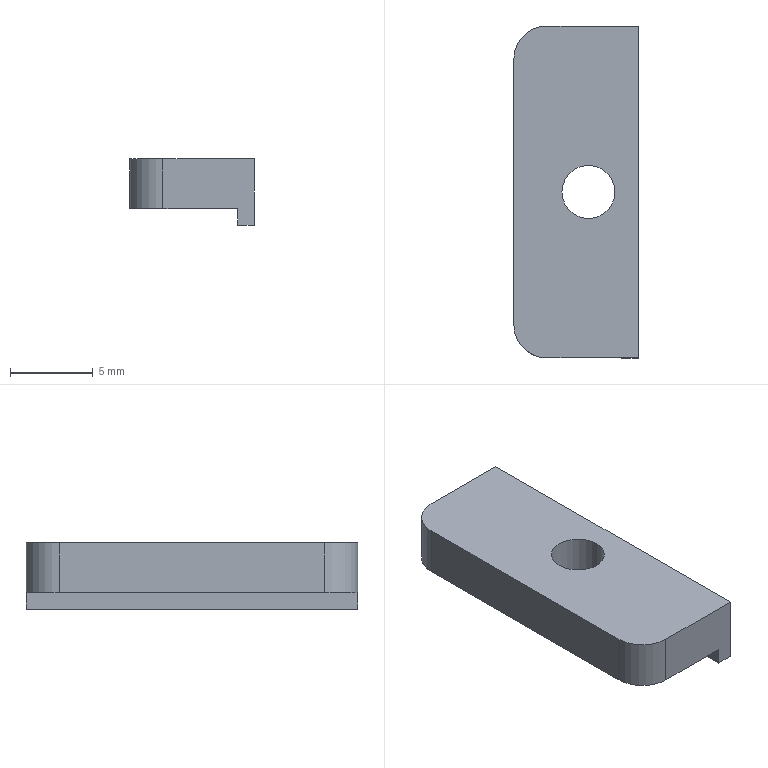Part | STEP file | PN_0043 Mount electronic clip pressure block A | 1 solid | 12 faces | box 7.5 x 20 x 4 mm | volume 440.722 mm3 | plane 8 | cylinder 4 | commonest cylinder face diameters 3.2 x2 4 x2
STEP:
#1=CARTESIAN_POINT('',(0.,0.,0.));
#2=DIRECTION('',(0.,0.,1.));
#3=DIRECTION('',(1.,0.,0.));
#4=AXIS2_PLACEMENT_3D('',#1,#2,#3);
#5=CARTESIAN_POINT('',(2.35,0.,1.));
#6=VERTEX_POINT('',#5);
#7=CARTESIAN_POINT('',(2.35,0.,4.));
#8=VERTEX_POINT('',#7);
#9=CARTESIAN_POINT('',(2.35,0.,4.));
#10=DIRECTION('',(0.,0.,1.));
#11=VECTOR('',#10,1.);
#12=LINE('',#9,#11);
#13=CARTESIAN_POINT('',(0.75,0.,4.));
#14=DIRECTION('',(0.,0.,1.));
#15=DIRECTION('',(1.,0.,0.));
#16=AXIS2_PLACEMENT_3D('',#13,#14,#15);
#17=CYLINDRICAL_SURFACE('',#16,1.6);
#18=CARTESIAN_POINT('',(6.283,0.));
#19=DIRECTION('',(0.,1.));
#20=VECTOR('',#19,1.);
#21=LINE('',#18,#20);
#22=(GEOMETRIC_REPRESENTATION_CONTEXT(2)PARAMETRIC_REPRESENTATION_CONTEXT()REPRESENTATION_CONTEXT('',''));
#23=DEFINITIONAL_REPRESENTATION('',(#21),#22);
#24=PCURVE('',#17,#23);
#25=CARTESIAN_POINT('',(0.75,0.,4.));
#26=DIRECTION('',(0.,0.,1.));
#27=DIRECTION('',(1.,0.,0.));
#28=AXIS2_PLACEMENT_3D('',#25,#26,#27);
#29=CYLINDRICAL_SURFACE('',#28,1.6);
#30=CARTESIAN_POINT('',(0.,0.));
#31=DIRECTION('',(0.,1.));
#32=VECTOR('',#31,1.);
#33=LINE('',#30,#32);
#34=(GEOMETRIC_REPRESENTATION_CONTEXT(2)PARAMETRIC_REPRESENTATION_CONTEXT()REPRESENTATION_CONTEXT('',''));
#35=DEFINITIONAL_REPRESENTATION('',(#33),#34);
#36=PCURVE('',#29,#35);
#37=SURFACE_CURVE('',#12,(#24,#36),.PCURVE_S1.);
#38=EDGE_CURVE('',#6,#8,#37,.T.);
#39=ORIENTED_EDGE('',*,*,#38,.T.);
#40=CARTESIAN_POINT('',(-0.85,0.,4.));
#41=VERTEX_POINT('',#40);
#42=CARTESIAN_POINT('',(0.75,0.,4.));
#43=DIRECTION('',(0.,0.,1.));
#44=DIRECTION('',(1.,0.,0.));
#45=AXIS2_PLACEMENT_3D('',#42,#43,#44);
#46=CIRCLE('',#45,1.6);
#47=CARTESIAN_POINT('',(0.,0.));
#48=DIRECTION('',(1.,0.));
#49=VECTOR('',#48,1.);
#50=LINE('',#47,#49);
#51=(GEOMETRIC_REPRESENTATION_CONTEXT(2)PARAMETRIC_REPRESENTATION_CONTEXT()REPRESENTATION_CONTEXT('',''));
#52=DEFINITIONAL_REPRESENTATION('',(#50),#51);
#53=PCURVE('',#17,#52);
#54=CARTESIAN_POINT('',(0.,0.,4.));
#55=DIRECTION('',(0.,0.,-1.));
#56=DIRECTION('',(-1.,0.,0.));
#57=AXIS2_PLACEMENT_3D('',#54,#55,#56);
#58=PLANE('',#57);
#59=CARTESIAN_POINT('',(-2.35,0.));
#60=CARTESIAN_POINT('',(-2.35,2.771));
#61=CARTESIAN_POINT('',(0.05,1.386));
#62=CARTESIAN_POINT('',(2.45,0.));
#63=CARTESIAN_POINT('',(0.05,-1.386));
#64=CARTESIAN_POINT('',(-2.35,-2.771));
#65=CARTESIAN_POINT('',(-2.35,0.));
#66=(BOUNDED_CURVE()B_SPLINE_CURVE(2,(#59,#60,#61,#62,#63,#64,#65),.UNSPECIFIED.,.T.,.F.)B_SPLINE_CURVE_WITH_KNOTS((1,2,2,2,2,1),(-2.094,0.,2.094,4.189,6.283,8.378),.UNSPECIFIED.)CURVE()GEOMETRIC_REPRESENTATION_ITEM()RATIONAL_B_SPLINE_CURVE((1.,0.5,1.,0.5,1.,0.5,1.))REPRESENTATION_ITEM(''));
#67=(GEOMETRIC_REPRESENTATION_CONTEXT(2)PARAMETRIC_REPRESENTATION_CONTEXT()REPRESENTATION_CONTEXT('',''));
#68=DEFINITIONAL_REPRESENTATION('',(#66),#67);
#69=PCURVE('',#58,#68);
#70=SURFACE_CURVE('',#46,(#53,#69),.PCURVE_S1.);
#71=EDGE_CURVE('',#41,#8,#70,.T.);
#72=ORIENTED_EDGE('',*,*,#71,.F.);
#73=CARTESIAN_POINT('',(-0.85,0.,1.));
#74=VERTEX_POINT('',#73);
#75=CARTESIAN_POINT('',(-0.85,0.,4.));
#76=DIRECTION('',(0.,0.,1.));
#77=VECTOR('',#76,1.);
#78=LINE('',#75,#77);
#79=CARTESIAN_POINT('',(3.142,0.));
#80=DIRECTION('',(0.,1.));
#81=VECTOR('',#80,1.);
#82=LINE('',#79,#81);
#83=(GEOMETRIC_REPRESENTATION_CONTEXT(2)PARAMETRIC_REPRESENTATION_CONTEXT()REPRESENTATION_CONTEXT('',''));
#84=DEFINITIONAL_REPRESENTATION('',(#82),#83);
#85=PCURVE('',#17,#84);
#86=CARTESIAN_POINT('',(3.142,0.));
#87=DIRECTION('',(0.,1.));
#88=VECTOR('',#87,1.);
#89=LINE('',#86,#88);
#90=(GEOMETRIC_REPRESENTATION_CONTEXT(2)PARAMETRIC_REPRESENTATION_CONTEXT()REPRESENTATION_CONTEXT('',''));
#91=DEFINITIONAL_REPRESENTATION('',(#89),#90);
#92=PCURVE('',#29,#91);
#93=SURFACE_CURVE('',#78,(#85,#92),.PCURVE_S1.);
#94=EDGE_CURVE('',#74,#41,#93,.T.);
#95=ORIENTED_EDGE('',*,*,#94,.F.);
#96=CARTESIAN_POINT('',(0.75,0.,1.));
#97=DIRECTION('',(0.,0.,1.));
#98=DIRECTION('',(1.,0.,0.));
#99=AXIS2_PLACEMENT_3D('',#96,#97,#98);
#100=CIRCLE('',#99,1.6);
#101=CARTESIAN_POINT('',(0.,-3.));
#102=DIRECTION('',(1.,0.));
#103=VECTOR('',#102,1.);
#104=LINE('',#101,#103);
#105=(GEOMETRIC_REPRESENTATION_CONTEXT(2)PARAMETRIC_REPRESENTATION_CONTEXT()REPRESENTATION_CONTEXT('',''));
#106=DEFINITIONAL_REPRESENTATION('',(#104),#105);
#107=PCURVE('',#17,#106);
#108=CARTESIAN_POINT('',(-3.75,10.,1.));
#109=DIRECTION('',(0.,0.,1.));
#110=DIRECTION('',(1.,0.,0.));
#111=AXIS2_PLACEMENT_3D('',#108,#109,#110);
#112=PLANE('',#111);
#113=CARTESIAN_POINT('',(4.5,-10.));
#114=DIRECTION('',(1.,0.));
#115=AXIS2_PLACEMENT_2D('',#113,#114);
#116=CIRCLE('',#115,1.6);
#117=(GEOMETRIC_REPRESENTATION_CONTEXT(2)PARAMETRIC_REPRESENTATION_CONTEXT()REPRESENTATION_CONTEXT('',''));
#118=DEFINITIONAL_REPRESENTATION('',(#116),#117);
#119=PCURVE('',#112,#118);
#120=SURFACE_CURVE('',#100,(#107,#119),.PCURVE_S1.);
#121=EDGE_CURVE('',#74,#6,#120,.T.);
#122=ORIENTED_EDGE('',*,*,#121,.T.);
#123=EDGE_LOOP('',(#39,#72,#95,#122));
#124=FACE_BOUND('',#123,.F.);
#125=ADVANCED_FACE('',(#124),#17,.F.);
#126=CARTESIAN_POINT('',(3.75,-10.,0.));
#127=VERTEX_POINT('',#126);
#128=CARTESIAN_POINT('',(3.75,10.,0.));
#129=VERTEX_POINT('',#128);
#130=CARTESIAN_POINT('',(3.75,-10.,0.));
#131=DIRECTION('',(0.,1.,0.));
#132=VECTOR('',#131,1.);
#133=LINE('',#130,#132);
#134=CARTESIAN_POINT('',(3.75,-10.,4.));
#135=DIRECTION('',(-1.,0.,0.));
#136=DIRECTION('',(0.,0.,1.));
#137=AXIS2_PLACEMENT_3D('',#134,#135,#136);
#138=PLANE('',#137);
#139=CARTESIAN_POINT('',(-4.,0.));
#140=DIRECTION('',(0.,1.));
#141=VECTOR('',#140,1.);
#142=LINE('',#139,#141);
#143=(GEOMETRIC_REPRESENTATION_CONTEXT(2)PARAMETRIC_REPRESENTATION_CONTEXT()REPRESENTATION_CONTEXT('',''));
#144=DEFINITIONAL_REPRESENTATION('',(#142),#143);
#145=PCURVE('',#138,#144);
#146=CARTESIAN_POINT('',(0.,0.,0.));
#147=DIRECTION('',(0.,0.,-1.));
#148=DIRECTION('',(-1.,0.,0.));
#149=AXIS2_PLACEMENT_3D('',#146,#147,#148);
#150=PLANE('',#149);
#151=CARTESIAN_POINT('',(-3.75,-10.));
#152=DIRECTION('',(0.,1.));
#153=VECTOR('',#152,1.);
#154=LINE('',#151,#153);
#155=(GEOMETRIC_REPRESENTATION_CONTEXT(2)PARAMETRIC_REPRESENTATION_CONTEXT()REPRESENTATION_CONTEXT('',''));
#156=DEFINITIONAL_REPRESENTATION('',(#154),#155);
#157=PCURVE('',#150,#156);
#158=SURFACE_CURVE('',#133,(#145,#157),.PCURVE_S1.);
#159=EDGE_CURVE('',#127,#129,#158,.T.);
#160=ORIENTED_EDGE('',*,*,#159,.T.);
#161=CARTESIAN_POINT('',(3.75,10.,4.));
#162=VERTEX_POINT('',#161);
#163=CARTESIAN_POINT('',(3.75,10.,4.));
#164=DIRECTION('',(0.,0.,-1.));
#165=VECTOR('',#164,1.);
#166=LINE('',#163,#165);
#167=CARTESIAN_POINT('',(0.,20.));
#168=DIRECTION('',(-1.,0.));
#169=VECTOR('',#168,1.);
#170=LINE('',#167,#169);
#171=(GEOMETRIC_REPRESENTATION_CONTEXT(2)PARAMETRIC_REPRESENTATION_CONTEXT()REPRESENTATION_CONTEXT('',''));
#172=DEFINITIONAL_REPRESENTATION('',(#170),#171);
#173=PCURVE('',#138,#172);
#174=CARTESIAN_POINT('',(-3.75,10.,4.));
#175=DIRECTION('',(0.,-1.,0.));
#176=DIRECTION('',(0.,0.,-1.));
#177=AXIS2_PLACEMENT_3D('',#174,#175,#176);
#178=PLANE('',#177);
#179=CARTESIAN_POINT('',(0.,7.5));
#180=DIRECTION('',(1.,0.));
#181=VECTOR('',#180,1.);
#182=LINE('',#179,#181);
#183=(GEOMETRIC_REPRESENTATION_CONTEXT(2)PARAMETRIC_REPRESENTATION_CONTEXT()REPRESENTATION_CONTEXT('',''));
#184=DEFINITIONAL_REPRESENTATION('',(#182),#183);
#185=PCURVE('',#178,#184);
#186=SURFACE_CURVE('',#166,(#173,#185),.PCURVE_S1.);
#187=EDGE_CURVE('',#162,#129,#186,.T.);
#188=ORIENTED_EDGE('',*,*,#187,.F.);
#189=CARTESIAN_POINT('',(3.75,-10.,4.));
#190=VERTEX_POINT('',#189);
#191=CARTESIAN_POINT('',(3.75,-10.,4.));
#192=DIRECTION('',(0.,1.,0.));
#193=VECTOR('',#192,1.);
#194=LINE('',#191,#193);
#195=CARTESIAN_POINT('',(0.,0.));
#196=DIRECTION('',(0.,1.));
#197=VECTOR('',#196,1.);
#198=LINE('',#195,#197);
#199=(GEOMETRIC_REPRESENTATION_CONTEXT(2)PARAMETRIC_REPRESENTATION_CONTEXT()REPRESENTATION_CONTEXT('',''));
#200=DEFINITIONAL_REPRESENTATION('',(#198),#199);
#201=PCURVE('',#138,#200);
#202=CARTESIAN_POINT('',(-3.75,-10.));
#203=DIRECTION('',(0.,1.));
#204=VECTOR('',#203,1.);
#205=LINE('',#202,#204);
#206=(GEOMETRIC_REPRESENTATION_CONTEXT(2)PARAMETRIC_REPRESENTATION_CONTEXT()REPRESENTATION_CONTEXT('',''));
#207=DEFINITIONAL_REPRESENTATION('',(#205),#206);
#208=PCURVE('',#58,#207);
#209=SURFACE_CURVE('',#194,(#201,#208),.PCURVE_S1.);
#210=EDGE_CURVE('',#190,#162,#209,.T.);
#211=ORIENTED_EDGE('',*,*,#210,.F.);
#212=CARTESIAN_POINT('',(3.75,-10.,4.));
#213=DIRECTION('',(0.,0.,-1.));
#214=VECTOR('',#213,1.);
#215=LINE('',#212,#214);
#216=CARTESIAN_POINT('',(0.,0.));
#217=DIRECTION('',(-1.,0.));
#218=VECTOR('',#217,1.);
#219=LINE('',#216,#218);
#220=(GEOMETRIC_REPRESENTATION_CONTEXT(2)PARAMETRIC_REPRESENTATION_CONTEXT()REPRESENTATION_CONTEXT('',''));
#221=DEFINITIONAL_REPRESENTATION('',(#219),#220);
#222=PCURVE('',#138,#221);
#223=CARTESIAN_POINT('',(-3.75,-10.,4.));
#224=DIRECTION('',(0.,1.,0.));
#225=DIRECTION('',(0.,0.,1.));
#226=AXIS2_PLACEMENT_3D('',#223,#224,#225);
#227=PLANE('',#226);
#228=CARTESIAN_POINT('',(0.,7.5));
#229=DIRECTION('',(-1.,0.));
#230=VECTOR('',#229,1.);
#231=LINE('',#228,#230);
#232=(GEOMETRIC_REPRESENTATION_CONTEXT(2)PARAMETRIC_REPRESENTATION_CONTEXT()REPRESENTATION_CONTEXT('',''));
#233=DEFINITIONAL_REPRESENTATION('',(#231),#232);
#234=PCURVE('',#227,#233);
#235=SURFACE_CURVE('',#215,(#222,#234),.PCURVE_S1.);
#236=EDGE_CURVE('',#190,#127,#235,.T.);
#237=ORIENTED_EDGE('',*,*,#236,.T.);
#238=EDGE_LOOP('',(#160,#188,#211,#237));
#239=FACE_BOUND('',#238,.T.);
#240=ADVANCED_FACE('',(#239),#138,.F.);
#241=CARTESIAN_POINT('',(2.75,10.,1.));
#242=VERTEX_POINT('',#241);
#243=CARTESIAN_POINT('',(-1.75,10.,1.));
#244=VERTEX_POINT('',#243);
#245=CARTESIAN_POINT('',(-3.75,10.,1.));
#246=DIRECTION('',(-1.,0.,0.));
#247=VECTOR('',#246,1.);
#248=LINE('',#245,#247);
#249=CARTESIAN_POINT('',(3.,0.));
#250=DIRECTION('',(0.,-1.));
#251=VECTOR('',#250,1.);
#252=LINE('',#249,#251);
#253=(GEOMETRIC_REPRESENTATION_CONTEXT(2)PARAMETRIC_REPRESENTATION_CONTEXT()REPRESENTATION_CONTEXT('',''));
#254=DEFINITIONAL_REPRESENTATION('',(#252),#253);
#255=PCURVE('',#178,#254);
#256=CARTESIAN_POINT('',(0.,0.));
#257=DIRECTION('',(-1.,0.));
#258=VECTOR('',#257,1.);
#259=LINE('',#256,#258);
#260=(GEOMETRIC_REPRESENTATION_CONTEXT(2)PARAMETRIC_REPRESENTATION_CONTEXT()REPRESENTATION_CONTEXT('',''));
#261=DEFINITIONAL_REPRESENTATION('',(#259),#260);
#262=PCURVE('',#112,#261);
#263=SURFACE_CURVE('',#248,(#255,#262),.PCURVE_S1.);
#264=EDGE_CURVE('',#242,#244,#263,.T.);
#265=ORIENTED_EDGE('',*,*,#264,.T.);
#266=CARTESIAN_POINT('',(-1.75,10.,4.));
#267=VERTEX_POINT('',#266);
#268=CARTESIAN_POINT('',(-1.75,10.,4.));
#269=DIRECTION('',(0.,0.,1.));
#270=VECTOR('',#269,1.);
#271=LINE('',#268,#270);
#272=CARTESIAN_POINT('',(0.,2.));
#273=DIRECTION('',(-1.,0.));
#274=VECTOR('',#273,1.);
#275=LINE('',#272,#274);
#276=(GEOMETRIC_REPRESENTATION_CONTEXT(2)PARAMETRIC_REPRESENTATION_CONTEXT()REPRESENTATION_CONTEXT('',''));
#277=DEFINITIONAL_REPRESENTATION('',(#275),#276);
#278=PCURVE('',#178,#277);
#279=CARTESIAN_POINT('',(-1.75,8.,4.));
#280=DIRECTION('',(0.,0.,-1.));
#281=DIRECTION('',(-1.,0.,0.));
#282=AXIS2_PLACEMENT_3D('',#279,#280,#281);
#283=CYLINDRICAL_SURFACE('',#282,2.);
#284=CARTESIAN_POINT('',(1.571,0.));
#285=DIRECTION('',(0.,-1.));
#286=VECTOR('',#285,1.);
#287=LINE('',#284,#286);
#288=(GEOMETRIC_REPRESENTATION_CONTEXT(2)PARAMETRIC_REPRESENTATION_CONTEXT()REPRESENTATION_CONTEXT('',''));
#289=DEFINITIONAL_REPRESENTATION('',(#287),#288);
#290=PCURVE('',#283,#289);
#291=SURFACE_CURVE('',#271,(#278,#290),.PCURVE_S1.);
#292=EDGE_CURVE('',#244,#267,#291,.T.);
#293=ORIENTED_EDGE('',*,*,#292,.T.);
#294=CARTESIAN_POINT('',(-3.75,10.,4.));
#295=DIRECTION('',(-1.,0.,0.));
#296=VECTOR('',#295,1.);
#297=LINE('',#294,#296);
#298=CARTESIAN_POINT('',(0.,0.));
#299=DIRECTION('',(0.,-1.));
#300=VECTOR('',#299,1.);
#301=LINE('',#298,#300);
#302=(GEOMETRIC_REPRESENTATION_CONTEXT(2)PARAMETRIC_REPRESENTATION_CONTEXT()REPRESENTATION_CONTEXT('',''));
#303=DEFINITIONAL_REPRESENTATION('',(#301),#302);
#304=PCURVE('',#178,#303);
#305=CARTESIAN_POINT('',(3.75,10.));
#306=DIRECTION('',(1.,0.));
#307=VECTOR('',#306,1.);
#308=LINE('',#305,#307);
#309=(GEOMETRIC_REPRESENTATION_CONTEXT(2)PARAMETRIC_REPRESENTATION_CONTEXT()REPRESENTATION_CONTEXT('',''));
#310=DEFINITIONAL_REPRESENTATION('',(#308),#309);
#311=PCURVE('',#58,#310);
#312=SURFACE_CURVE('',#297,(#304,#311),.PCURVE_S1.);
#313=EDGE_CURVE('',#162,#267,#312,.T.);
#314=ORIENTED_EDGE('',*,*,#313,.F.);
#315=ORIENTED_EDGE('',*,*,#187,.T.);
#316=CARTESIAN_POINT('',(2.75,10.,0.));
#317=VERTEX_POINT('',#316);
#318=CARTESIAN_POINT('',(-3.75,10.,0.));
#319=DIRECTION('',(-1.,0.,0.));
#320=VECTOR('',#319,1.);
#321=LINE('',#318,#320);
#322=CARTESIAN_POINT('',(4.,0.));
#323=DIRECTION('',(0.,-1.));
#324=VECTOR('',#323,1.);
#325=LINE('',#322,#324);
#326=(GEOMETRIC_REPRESENTATION_CONTEXT(2)PARAMETRIC_REPRESENTATION_CONTEXT()REPRESENTATION_CONTEXT('',''));
#327=DEFINITIONAL_REPRESENTATION('',(#325),#326);
#328=PCURVE('',#178,#327);
#329=CARTESIAN_POINT('',(3.75,10.));
#330=DIRECTION('',(1.,0.));
#331=VECTOR('',#330,1.);
#332=LINE('',#329,#331);
#333=(GEOMETRIC_REPRESENTATION_CONTEXT(2)PARAMETRIC_REPRESENTATION_CONTEXT()REPRESENTATION_CONTEXT('',''));
#334=DEFINITIONAL_REPRESENTATION('',(#332),#333);
#335=PCURVE('',#150,#334);
#336=SURFACE_CURVE('',#321,(#328,#335),.PCURVE_S1.);
#337=EDGE_CURVE('',#129,#317,#336,.T.);
#338=ORIENTED_EDGE('',*,*,#337,.T.);
#339=CARTESIAN_POINT('',(2.75,10.,0.));
#340=DIRECTION('',(0.,0.,1.));
#341=VECTOR('',#340,1.);
#342=LINE('',#339,#341);
#343=CARTESIAN_POINT('',(4.,6.5));
#344=DIRECTION('',(-1.,0.));
#345=VECTOR('',#344,1.);
#346=LINE('',#343,#345);
#347=(GEOMETRIC_REPRESENTATION_CONTEXT(2)PARAMETRIC_REPRESENTATION_CONTEXT()REPRESENTATION_CONTEXT('',''));
#348=DEFINITIONAL_REPRESENTATION('',(#346),#347);
#349=PCURVE('',#178,#348);
#350=CARTESIAN_POINT('',(2.75,10.,0.));
#351=DIRECTION('',(1.,0.,0.));
#352=DIRECTION('',(0.,0.,-1.));
#353=AXIS2_PLACEMENT_3D('',#350,#351,#352);
#354=PLANE('',#353);
#355=CARTESIAN_POINT('',(0.,0.));
#356=DIRECTION('',(-1.,0.));
#357=VECTOR('',#356,1.);
#358=LINE('',#355,#357);
#359=(GEOMETRIC_REPRESENTATION_CONTEXT(2)PARAMETRIC_REPRESENTATION_CONTEXT()REPRESENTATION_CONTEXT('',''));
#360=DEFINITIONAL_REPRESENTATION('',(#358),#359);
#361=PCURVE('',#354,#360);
#362=SURFACE_CURVE('',#342,(#349,#361),.PCURVE_S1.);
#363=EDGE_CURVE('',#317,#242,#362,.T.);
#364=ORIENTED_EDGE('',*,*,#363,.T.);
#365=EDGE_LOOP('',(#265,#293,#314,#315,#338,#364));
#366=FACE_BOUND('',#365,.T.);
#367=ADVANCED_FACE('',(#366),#178,.F.);
#368=CARTESIAN_POINT('',(-3.75,8.,4.));
#369=VERTEX_POINT('',#368);
#370=CARTESIAN_POINT('',(-3.75,-8.,4.));
#371=VERTEX_POINT('',#370);
#372=CARTESIAN_POINT('',(-3.75,-10.,4.));
#373=DIRECTION('',(0.,-1.,0.));
#374=VECTOR('',#373,1.);
#375=LINE('',#372,#374);
#376=CARTESIAN_POINT('',(-3.75,-10.,4.));
#377=DIRECTION('',(1.,0.,0.));
#378=DIRECTION('',(0.,0.,-1.));
#379=AXIS2_PLACEMENT_3D('',#376,#377,#378);
#380=PLANE('',#379);
#381=CARTESIAN_POINT('',(0.,0.));
#382=DIRECTION('',(0.,-1.));
#383=VECTOR('',#382,1.);
#384=LINE('',#381,#383);
#385=(GEOMETRIC_REPRESENTATION_CONTEXT(2)PARAMETRIC_REPRESENTATION_CONTEXT()REPRESENTATION_CONTEXT('',''));
#386=DEFINITIONAL_REPRESENTATION('',(#384),#385);
#387=PCURVE('',#380,#386);
#388=CARTESIAN_POINT('',(3.75,-10.));
#389=DIRECTION('',(0.,-1.));
#390=VECTOR('',#389,1.);
#391=LINE('',#388,#390);
#392=(GEOMETRIC_REPRESENTATION_CONTEXT(2)PARAMETRIC_REPRESENTATION_CONTEXT()REPRESENTATION_CONTEXT('',''));
#393=DEFINITIONAL_REPRESENTATION('',(#391),#392);
#394=PCURVE('',#58,#393);
#395=SURFACE_CURVE('',#375,(#387,#394),.PCURVE_S1.);
#396=EDGE_CURVE('',#369,#371,#395,.T.);
#397=ORIENTED_EDGE('',*,*,#396,.F.);
#398=CARTESIAN_POINT('',(-3.75,8.,1.));
#399=VERTEX_POINT('',#398);
#400=CARTESIAN_POINT('',(-3.75,8.,4.));
#401=DIRECTION('',(0.,0.,-1.));
#402=VECTOR('',#401,1.);
#403=LINE('',#400,#402);
#404=CARTESIAN_POINT('',(0.,18.));
#405=DIRECTION('',(1.,0.));
#406=VECTOR('',#405,1.);
#407=LINE('',#404,#406);
#408=(GEOMETRIC_REPRESENTATION_CONTEXT(2)PARAMETRIC_REPRESENTATION_CONTEXT()REPRESENTATION_CONTEXT('',''));
#409=DEFINITIONAL_REPRESENTATION('',(#407),#408);
#410=PCURVE('',#380,#409);
#411=CARTESIAN_POINT('',(0.,0.));
#412=DIRECTION('',(0.,1.));
#413=VECTOR('',#412,1.);
#414=LINE('',#411,#413);
#415=(GEOMETRIC_REPRESENTATION_CONTEXT(2)PARAMETRIC_REPRESENTATION_CONTEXT()REPRESENTATION_CONTEXT('',''));
#416=DEFINITIONAL_REPRESENTATION('',(#414),#415);
#417=PCURVE('',#283,#416);
#418=SURFACE_CURVE('',#403,(#410,#417),.PCURVE_S1.);
#419=EDGE_CURVE('',#369,#399,#418,.T.);
#420=ORIENTED_EDGE('',*,*,#419,.T.);
#421=CARTESIAN_POINT('',(-3.75,-8.,1.));
#422=VERTEX_POINT('',#421);
#423=CARTESIAN_POINT('',(-3.75,10.,1.));
#424=DIRECTION('',(0.,-1.,0.));
#425=VECTOR('',#424,1.);
#426=LINE('',#423,#425);
#427=CARTESIAN_POINT('',(3.,20.));
#428=DIRECTION('',(0.,-1.));
#429=VECTOR('',#428,1.);
#430=LINE('',#427,#429);
#431=(GEOMETRIC_REPRESENTATION_CONTEXT(2)PARAMETRIC_REPRESENTATION_CONTEXT()REPRESENTATION_CONTEXT('',''));
#432=DEFINITIONAL_REPRESENTATION('',(#430),#431);
#433=PCURVE('',#380,#432);
#434=CARTESIAN_POINT('',(0.,0.));
#435=DIRECTION('',(0.,-1.));
#436=VECTOR('',#435,1.);
#437=LINE('',#434,#436);
#438=(GEOMETRIC_REPRESENTATION_CONTEXT(2)PARAMETRIC_REPRESENTATION_CONTEXT()REPRESENTATION_CONTEXT('',''));
#439=DEFINITIONAL_REPRESENTATION('',(#437),#438);
#440=PCURVE('',#112,#439);
#441=SURFACE_CURVE('',#426,(#433,#440),.PCURVE_S1.);
#442=EDGE_CURVE('',#399,#422,#441,.T.);
#443=ORIENTED_EDGE('',*,*,#442,.T.);
#444=CARTESIAN_POINT('',(-3.75,-8.,4.));
#445=DIRECTION('',(0.,0.,1.));
#446=VECTOR('',#445,1.);
#447=LINE('',#444,#446);
#448=CARTESIAN_POINT('',(0.,2.));
#449=DIRECTION('',(-1.,0.));
#450=VECTOR('',#449,1.);
#451=LINE('',#448,#450);
#452=(GEOMETRIC_REPRESENTATION_CONTEXT(2)PARAMETRIC_REPRESENTATION_CONTEXT()REPRESENTATION_CONTEXT('',''));
#453=DEFINITIONAL_REPRESENTATION('',(#451),#452);
#454=PCURVE('',#380,#453);
#455=CARTESIAN_POINT('',(-1.75,-8.,4.));
#456=DIRECTION('',(0.,0.,-1.));
#457=DIRECTION('',(-1.,0.,0.));
#458=AXIS2_PLACEMENT_3D('',#455,#456,#457);
#459=CYLINDRICAL_SURFACE('',#458,2.);
#460=CARTESIAN_POINT('',(6.283,0.));
#461=DIRECTION('',(0.,-1.));
#462=VECTOR('',#461,1.);
#463=LINE('',#460,#462);
#464=(GEOMETRIC_REPRESENTATION_CONTEXT(2)PARAMETRIC_REPRESENTATION_CONTEXT()REPRESENTATION_CONTEXT('',''));
#465=DEFINITIONAL_REPRESENTATION('',(#463),#464);
#466=PCURVE('',#459,#465);
#467=SURFACE_CURVE('',#447,(#454,#466),.PCURVE_S1.);
#468=EDGE_CURVE('',#422,#371,#467,.T.);
#469=ORIENTED_EDGE('',*,*,#468,.T.);
#470=EDGE_LOOP('',(#397,#420,#443,#469));
#471=FACE_BOUND('',#470,.T.);
#472=ADVANCED_FACE('',(#471),#380,.F.);
#473=CARTESIAN_POINT('',(-1.75,-10.,4.));
#474=VERTEX_POINT('',#473);
#475=CARTESIAN_POINT('',(-3.75,-10.,4.));
#476=DIRECTION('',(1.,0.,0.));
#477=VECTOR('',#476,1.);
#478=LINE('',#475,#477);
#479=CARTESIAN_POINT('',(0.,0.));
#480=DIRECTION('',(0.,1.));
#481=VECTOR('',#480,1.);
#482=LINE('',#479,#481);
#483=(GEOMETRIC_REPRESENTATION_CONTEXT(2)PARAMETRIC_REPRESENTATION_CONTEXT()REPRESENTATION_CONTEXT('',''));
#484=DEFINITIONAL_REPRESENTATION('',(#482),#483);
#485=PCURVE('',#227,#484);
#486=CARTESIAN_POINT('',(3.75,-10.));
#487=DIRECTION('',(-1.,0.));
#488=VECTOR('',#487,1.);
#489=LINE('',#486,#488);
#490=(GEOMETRIC_REPRESENTATION_CONTEXT(2)PARAMETRIC_REPRESENTATION_CONTEXT()REPRESENTATION_CONTEXT('',''));
#491=DEFINITIONAL_REPRESENTATION('',(#489),#490);
#492=PCURVE('',#58,#491);
#493=SURFACE_CURVE('',#478,(#485,#492),.PCURVE_S1.);
#494=EDGE_CURVE('',#474,#190,#493,.T.);
#495=ORIENTED_EDGE('',*,*,#494,.F.);
#496=CARTESIAN_POINT('',(-1.75,-10.,1.));
#497=VERTEX_POINT('',#496);
#498=CARTESIAN_POINT('',(-1.75,-10.,4.));
#499=DIRECTION('',(0.,0.,-1.));
#500=VECTOR('',#499,1.);
#501=LINE('',#498,#500);
#502=CARTESIAN_POINT('',(0.,2.));
#503=DIRECTION('',(-1.,0.));
#504=VECTOR('',#503,1.);
#505=LINE('',#502,#504);
#506=(GEOMETRIC_REPRESENTATION_CONTEXT(2)PARAMETRIC_REPRESENTATION_CONTEXT()REPRESENTATION_CONTEXT('',''));
#507=DEFINITIONAL_REPRESENTATION('',(#505),#506);
#508=PCURVE('',#227,#507);
#509=CARTESIAN_POINT('',(4.712,0.));
#510=DIRECTION('',(0.,1.));
#511=VECTOR('',#510,1.);
#512=LINE('',#509,#511);
#513=(GEOMETRIC_REPRESENTATION_CONTEXT(2)PARAMETRIC_REPRESENTATION_CONTEXT()REPRESENTATION_CONTEXT('',''));
#514=DEFINITIONAL_REPRESENTATION('',(#512),#513);
#515=PCURVE('',#459,#514);
#516=SURFACE_CURVE('',#501,(#508,#515),.PCURVE_S1.);
#517=EDGE_CURVE('',#474,#497,#516,.T.);
#518=ORIENTED_EDGE('',*,*,#517,.T.);
#519=CARTESIAN_POINT('',(2.75,-10.,1.));
#520=VERTEX_POINT('',#519);
#521=CARTESIAN_POINT('',(-3.75,-10.,1.));
#522=DIRECTION('',(-1.,0.,0.));
#523=VECTOR('',#522,1.);
#524=LINE('',#521,#523);
#525=CARTESIAN_POINT('',(-3.,0.));
#526=DIRECTION('',(0.,-1.));
#527=VECTOR('',#526,1.);
#528=LINE('',#525,#527);
#529=(GEOMETRIC_REPRESENTATION_CONTEXT(2)PARAMETRIC_REPRESENTATION_CONTEXT()REPRESENTATION_CONTEXT('',''));
#530=DEFINITIONAL_REPRESENTATION('',(#528),#529);
#531=PCURVE('',#227,#530);
#532=CARTESIAN_POINT('',(0.,-20.));
#533=DIRECTION('',(-1.,0.));
#534=VECTOR('',#533,1.);
#535=LINE('',#532,#534);
#536=(GEOMETRIC_REPRESENTATION_CONTEXT(2)PARAMETRIC_REPRESENTATION_CONTEXT()REPRESENTATION_CONTEXT('',''));
#537=DEFINITIONAL_REPRESENTATION('',(#535),#536);
#538=PCURVE('',#112,#537);
#539=SURFACE_CURVE('',#524,(#531,#538),.PCURVE_S1.);
#540=EDGE_CURVE('',#520,#497,#539,.T.);
#541=ORIENTED_EDGE('',*,*,#540,.F.);
#542=CARTESIAN_POINT('',(2.75,-10.,0.));
#543=VERTEX_POINT('',#542);
#544=CARTESIAN_POINT('',(2.75,-10.,0.));
#545=DIRECTION('',(0.,0.,1.));
#546=VECTOR('',#545,1.);
#547=LINE('',#544,#546);
#548=CARTESIAN_POINT('',(-4.,6.5));
#549=DIRECTION('',(1.,0.));
#550=VECTOR('',#549,1.);
#551=LINE('',#548,#550);
#552=(GEOMETRIC_REPRESENTATION_CONTEXT(2)PARAMETRIC_REPRESENTATION_CONTEXT()REPRESENTATION_CONTEXT('',''));
#553=DEFINITIONAL_REPRESENTATION('',(#551),#552);
#554=PCURVE('',#227,#553);
#555=CARTESIAN_POINT('',(0.,-20.));
#556=DIRECTION('',(-1.,0.));
#557=VECTOR('',#556,1.);
#558=LINE('',#555,#557);
#559=(GEOMETRIC_REPRESENTATION_CONTEXT(2)PARAMETRIC_REPRESENTATION_CONTEXT()REPRESENTATION_CONTEXT('',''));
#560=DEFINITIONAL_REPRESENTATION('',(#558),#559);
#561=PCURVE('',#354,#560);
#562=SURFACE_CURVE('',#547,(#554,#561),.PCURVE_S1.);
#563=EDGE_CURVE('',#543,#520,#562,.T.);
#564=ORIENTED_EDGE('',*,*,#563,.F.);
#565=CARTESIAN_POINT('',(-3.75,-10.,0.));
#566=DIRECTION('',(1.,0.,0.));
#567=VECTOR('',#566,1.);
#568=LINE('',#565,#567);
#569=CARTESIAN_POINT('',(-4.,0.));
#570=DIRECTION('',(0.,1.));
#571=VECTOR('',#570,1.);
#572=LINE('',#569,#571);
#573=(GEOMETRIC_REPRESENTATION_CONTEXT(2)PARAMETRIC_REPRESENTATION_CONTEXT()REPRESENTATION_CONTEXT('',''));
#574=DEFINITIONAL_REPRESENTATION('',(#572),#573);
#575=PCURVE('',#227,#574);
#576=CARTESIAN_POINT('',(3.75,-10.));
#577=DIRECTION('',(-1.,0.));
#578=VECTOR('',#577,1.);
#579=LINE('',#576,#578);
#580=(GEOMETRIC_REPRESENTATION_CONTEXT(2)PARAMETRIC_REPRESENTATION_CONTEXT()REPRESENTATION_CONTEXT('',''));
#581=DEFINITIONAL_REPRESENTATION('',(#579),#580);
#582=PCURVE('',#150,#581);
#583=SURFACE_CURVE('',#568,(#575,#582),.PCURVE_S1.);
#584=EDGE_CURVE('',#543,#127,#583,.T.);
#585=ORIENTED_EDGE('',*,*,#584,.T.);
#586=ORIENTED_EDGE('',*,*,#236,.F.);
#587=EDGE_LOOP('',(#495,#518,#541,#564,#585,#586));
#588=FACE_BOUND('',#587,.T.);
#589=ADVANCED_FACE('',(#588),#227,.F.);
#590=CARTESIAN_POINT('',(0.75,0.,4.));
#591=DIRECTION('',(0.,0.,1.));
#592=DIRECTION('',(1.,0.,0.));
#593=AXIS2_PLACEMENT_3D('',#590,#591,#592);
#594=CIRCLE('',#593,1.6);
#595=CARTESIAN_POINT('',(-2.35,0.));
#596=CARTESIAN_POINT('',(-2.35,2.771));
#597=CARTESIAN_POINT('',(0.05,1.386));
#598=CARTESIAN_POINT('',(2.45,0.));
#599=CARTESIAN_POINT('',(0.05,-1.386));
#600=CARTESIAN_POINT('',(-2.35,-2.771));
#601=CARTESIAN_POINT('',(-2.35,0.));
#602=(BOUNDED_CURVE()B_SPLINE_CURVE(2,(#595,#596,#597,#598,#599,#600,#601),.UNSPECIFIED.,.T.,.F.)B_SPLINE_CURVE_WITH_KNOTS((1,2,2,2,2,1),(-2.094,0.,2.094,4.189,6.283,8.378),.UNSPECIFIED.)CURVE()GEOMETRIC_REPRESENTATION_ITEM()RATIONAL_B_SPLINE_CURVE((1.,0.5,1.,0.5,1.,0.5,1.))REPRESENTATION_ITEM(''));
#603=(GEOMETRIC_REPRESENTATION_CONTEXT(2)PARAMETRIC_REPRESENTATION_CONTEXT()REPRESENTATION_CONTEXT('',''));
#604=DEFINITIONAL_REPRESENTATION('',(#602),#603);
#605=PCURVE('',#58,#604);
#606=CARTESIAN_POINT('',(0.,0.));
#607=DIRECTION('',(1.,0.));
#608=VECTOR('',#607,1.);
#609=LINE('',#606,#608);
#610=(GEOMETRIC_REPRESENTATION_CONTEXT(2)PARAMETRIC_REPRESENTATION_CONTEXT()REPRESENTATION_CONTEXT('',''));
#611=DEFINITIONAL_REPRESENTATION('',(#609),#610);
#612=PCURVE('',#29,#611);
#613=SURFACE_CURVE('',#594,(#605,#612),.PCURVE_S1.);
#614=EDGE_CURVE('',#8,#41,#613,.T.);
#615=ORIENTED_EDGE('',*,*,#614,.F.);
#616=ORIENTED_EDGE('',*,*,#71,.F.);
#617=EDGE_LOOP('',(#615,#616));
#618=FACE_BOUND('',#617,.T.);
#619=ORIENTED_EDGE('',*,*,#313,.T.);
#620=CARTESIAN_POINT('',(-1.75,8.,4.));
#621=DIRECTION('',(0.,0.,1.));
#622=DIRECTION('',(-1.,0.,0.));
#623=AXIS2_PLACEMENT_3D('',#620,#621,#622);
#624=CIRCLE('',#623,2.);
#625=CARTESIAN_POINT('',(3.75,8.));
#626=CARTESIAN_POINT('',(3.75,4.536));
#627=CARTESIAN_POINT('',(0.75,6.268));
#628=CARTESIAN_POINT('',(-2.25,8.));
#629=CARTESIAN_POINT('',(0.75,9.732));
#630=CARTESIAN_POINT('',(3.75,11.464));
#631=CARTESIAN_POINT('',(3.75,8.));
#632=(BOUNDED_CURVE()B_SPLINE_CURVE(2,(#625,#626,#627,#628,#629,#630,#631),.UNSPECIFIED.,.T.,.F.)B_SPLINE_CURVE_WITH_KNOTS((1,2,2,2,2,1),(-2.094,0.,2.094,4.189,6.283,8.378),.UNSPECIFIED.)CURVE()GEOMETRIC_REPRESENTATION_ITEM()RATIONAL_B_SPLINE_CURVE((1.,0.5,1.,0.5,1.,0.5,1.))REPRESENTATION_ITEM(''));
#633=(GEOMETRIC_REPRESENTATION_CONTEXT(2)PARAMETRIC_REPRESENTATION_CONTEXT()REPRESENTATION_CONTEXT('',''));
#634=DEFINITIONAL_REPRESENTATION('',(#632),#633);
#635=PCURVE('',#58,#634);
#636=CARTESIAN_POINT('',(6.283,0.));
#637=DIRECTION('',(-1.,0.));
#638=VECTOR('',#637,1.);
#639=LINE('',#636,#638);
#640=(GEOMETRIC_REPRESENTATION_CONTEXT(2)PARAMETRIC_REPRESENTATION_CONTEXT()REPRESENTATION_CONTEXT('',''));
#641=DEFINITIONAL_REPRESENTATION('',(#639),#640);
#642=PCURVE('',#283,#641);
#643=SURFACE_CURVE('',#624,(#635,#642),.PCURVE_S1.);
#644=EDGE_CURVE('',#267,#369,#643,.T.);
#645=ORIENTED_EDGE('',*,*,#644,.T.);
#646=ORIENTED_EDGE('',*,*,#396,.T.);
#647=CARTESIAN_POINT('',(-1.75,-8.,4.));
#648=DIRECTION('',(0.,0.,1.));
#649=DIRECTION('',(-1.,0.,0.));
#650=AXIS2_PLACEMENT_3D('',#647,#648,#649);
#651=CIRCLE('',#650,2.);
#652=CARTESIAN_POINT('',(3.75,-8.));
#653=CARTESIAN_POINT('',(3.75,-11.464));
#654=CARTESIAN_POINT('',(0.75,-9.732));
#655=CARTESIAN_POINT('',(-2.25,-8.));
#656=CARTESIAN_POINT('',(0.75,-6.268));
#657=CARTESIAN_POINT('',(3.75,-4.536));
#658=CARTESIAN_POINT('',(3.75,-8.));
#659=(BOUNDED_CURVE()B_SPLINE_CURVE(2,(#652,#653,#654,#655,#656,#657,#658),.UNSPECIFIED.,.T.,.F.)B_SPLINE_CURVE_WITH_KNOTS((1,2,2,2,2,1),(-2.094,0.,2.094,4.189,6.283,8.378),.UNSPECIFIED.)CURVE()GEOMETRIC_REPRESENTATION_ITEM()RATIONAL_B_SPLINE_CURVE((1.,0.5,1.,0.5,1.,0.5,1.))REPRESENTATION_ITEM(''));
#660=(GEOMETRIC_REPRESENTATION_CONTEXT(2)PARAMETRIC_REPRESENTATION_CONTEXT()REPRESENTATION_CONTEXT('',''));
#661=DEFINITIONAL_REPRESENTATION('',(#659),#660);
#662=PCURVE('',#58,#661);
#663=CARTESIAN_POINT('',(6.283,0.));
#664=DIRECTION('',(-1.,0.));
#665=VECTOR('',#664,1.);
#666=LINE('',#663,#665);
#667=(GEOMETRIC_REPRESENTATION_CONTEXT(2)PARAMETRIC_REPRESENTATION_CONTEXT()REPRESENTATION_CONTEXT('',''));
#668=DEFINITIONAL_REPRESENTATION('',(#666),#667);
#669=PCURVE('',#459,#668);
#670=SURFACE_CURVE('',#651,(#662,#669),.PCURVE_S1.);
#671=EDGE_CURVE('',#371,#474,#670,.T.);
#672=ORIENTED_EDGE('',*,*,#671,.T.);
#673=ORIENTED_EDGE('',*,*,#494,.T.);
#674=ORIENTED_EDGE('',*,*,#210,.T.);
#675=EDGE_LOOP('',(#619,#645,#646,#672,#673,#674));
#676=FACE_BOUND('',#675,.T.);
#677=ADVANCED_FACE('',(#618,#676),#58,.F.);
#678=CARTESIAN_POINT('',(2.75,10.,0.));
#679=DIRECTION('',(0.,-1.,0.));
#680=VECTOR('',#679,1.);
#681=LINE('',#678,#680);
#682=CARTESIAN_POINT('',(-2.75,10.));
#683=DIRECTION('',(0.,-1.));
#684=VECTOR('',#683,1.);
#685=LINE('',#682,#684);
#686=(GEOMETRIC_REPRESENTATION_CONTEXT(2)PARAMETRIC_REPRESENTATION_CONTEXT()REPRESENTATION_CONTEXT('',''));
#687=DEFINITIONAL_REPRESENTATION('',(#685),#686);
#688=PCURVE('',#150,#687);
#689=CARTESIAN_POINT('',(0.,0.));
#690=DIRECTION('',(0.,-1.));
#691=VECTOR('',#690,1.);
#692=LINE('',#689,#691);
#693=(GEOMETRIC_REPRESENTATION_CONTEXT(2)PARAMETRIC_REPRESENTATION_CONTEXT()REPRESENTATION_CONTEXT('',''));
#694=DEFINITIONAL_REPRESENTATION('',(#692),#693);
#695=PCURVE('',#354,#694);
#696=SURFACE_CURVE('',#681,(#688,#695),.PCURVE_S1.);
#697=EDGE_CURVE('',#317,#543,#696,.T.);
#698=ORIENTED_EDGE('',*,*,#697,.F.);
#699=ORIENTED_EDGE('',*,*,#337,.F.);
#700=ORIENTED_EDGE('',*,*,#159,.F.);
#701=ORIENTED_EDGE('',*,*,#584,.F.);
#702=EDGE_LOOP('',(#698,#699,#700,#701));
#703=FACE_BOUND('',#702,.T.);
#704=ADVANCED_FACE('',(#703),#150,.T.);
#705=CARTESIAN_POINT('',(0.75,0.,1.));
#706=DIRECTION('',(0.,0.,1.));
#707=DIRECTION('',(1.,0.,0.));
#708=AXIS2_PLACEMENT_3D('',#705,#706,#707);
#709=CIRCLE('',#708,1.6);
#710=CARTESIAN_POINT('',(4.5,-10.));
#711=DIRECTION('',(1.,0.));
#712=AXIS2_PLACEMENT_2D('',#710,#711);
#713=CIRCLE('',#712,1.6);
#714=(GEOMETRIC_REPRESENTATION_CONTEXT(2)PARAMETRIC_REPRESENTATION_CONTEXT()REPRESENTATION_CONTEXT('',''));
#715=DEFINITIONAL_REPRESENTATION('',(#713),#714);
#716=PCURVE('',#112,#715);
#717=CARTESIAN_POINT('',(0.,-3.));
#718=DIRECTION('',(1.,0.));
#719=VECTOR('',#718,1.);
#720=LINE('',#717,#719);
#721=(GEOMETRIC_REPRESENTATION_CONTEXT(2)PARAMETRIC_REPRESENTATION_CONTEXT()REPRESENTATION_CONTEXT('',''));
#722=DEFINITIONAL_REPRESENTATION('',(#720),#721);
#723=PCURVE('',#29,#722);
#724=SURFACE_CURVE('',#709,(#716,#723),.PCURVE_S1.);
#725=EDGE_CURVE('',#6,#74,#724,.T.);
#726=ORIENTED_EDGE('',*,*,#725,.T.);
#727=ORIENTED_EDGE('',*,*,#121,.T.);
#728=EDGE_LOOP('',(#726,#727));
#729=FACE_BOUND('',#728,.T.);
#730=ORIENTED_EDGE('',*,*,#442,.F.);
#731=CARTESIAN_POINT('',(-1.75,8.,1.));
#732=DIRECTION('',(0.,0.,-1.));
#733=DIRECTION('',(1.,0.,0.));
#734=AXIS2_PLACEMENT_3D('',#731,#732,#733);
#735=CIRCLE('',#734,2.);
#736=CARTESIAN_POINT('',(4.,-2.));
#737=CARTESIAN_POINT('',(4.,-5.464));
#738=CARTESIAN_POINT('',(1.,-3.732));
#739=CARTESIAN_POINT('',(-2.,-2.));
#740=CARTESIAN_POINT('',(1.,-0.2679));
#741=CARTESIAN_POINT('',(4.,1.464));
#742=CARTESIAN_POINT('',(4.,-2.));
#743=(BOUNDED_CURVE()B_SPLINE_CURVE(2,(#736,#737,#738,#739,#740,#741,#742),.UNSPECIFIED.,.T.,.F.)B_SPLINE_CURVE_WITH_KNOTS((1,2,2,2,2,1),(-2.094,0.,2.094,4.189,6.283,8.378),.UNSPECIFIED.)CURVE()GEOMETRIC_REPRESENTATION_ITEM()RATIONAL_B_SPLINE_CURVE((1.,0.5,1.,0.5,1.,0.5,1.))REPRESENTATION_ITEM(''));
#744=(GEOMETRIC_REPRESENTATION_CONTEXT(2)PARAMETRIC_REPRESENTATION_CONTEXT()REPRESENTATION_CONTEXT('',''));
#745=DEFINITIONAL_REPRESENTATION('',(#743),#744);
#746=PCURVE('',#112,#745);
#747=CARTESIAN_POINT('',(-3.142,3.));
#748=DIRECTION('',(1.,0.));
#749=VECTOR('',#748,1.);
#750=LINE('',#747,#749);
#751=(GEOMETRIC_REPRESENTATION_CONTEXT(2)PARAMETRIC_REPRESENTATION_CONTEXT()REPRESENTATION_CONTEXT('',''));
#752=DEFINITIONAL_REPRESENTATION('',(#750),#751);
#753=PCURVE('',#283,#752);
#754=SURFACE_CURVE('',#735,(#746,#753),.PCURVE_S1.);
#755=EDGE_CURVE('',#399,#244,#754,.T.);
#756=ORIENTED_EDGE('',*,*,#755,.T.);
#757=ORIENTED_EDGE('',*,*,#264,.F.);
#758=CARTESIAN_POINT('',(2.75,10.,1.));
#759=DIRECTION('',(0.,-1.,0.));
#760=VECTOR('',#759,1.);
#761=LINE('',#758,#760);
#762=CARTESIAN_POINT('',(6.5,0.));
#763=DIRECTION('',(0.,-1.));
#764=VECTOR('',#763,1.);
#765=LINE('',#762,#764);
#766=(GEOMETRIC_REPRESENTATION_CONTEXT(2)PARAMETRIC_REPRESENTATION_CONTEXT()REPRESENTATION_CONTEXT('',''));
#767=DEFINITIONAL_REPRESENTATION('',(#765),#766);
#768=PCURVE('',#112,#767);
#769=CARTESIAN_POINT('',(-1.,0.));
#770=DIRECTION('',(0.,-1.));
#771=VECTOR('',#770,1.);
#772=LINE('',#769,#771);
#773=(GEOMETRIC_REPRESENTATION_CONTEXT(2)PARAMETRIC_REPRESENTATION_CONTEXT()REPRESENTATION_CONTEXT('',''));
#774=DEFINITIONAL_REPRESENTATION('',(#772),#773);
#775=PCURVE('',#354,#774);
#776=SURFACE_CURVE('',#761,(#768,#775),.PCURVE_S1.);
#777=EDGE_CURVE('',#242,#520,#776,.T.);
#778=ORIENTED_EDGE('',*,*,#777,.T.);
#779=ORIENTED_EDGE('',*,*,#540,.T.);
#780=CARTESIAN_POINT('',(-1.75,-8.,1.));
#781=DIRECTION('',(0.,0.,-1.));
#782=DIRECTION('',(1.,0.,0.));
#783=AXIS2_PLACEMENT_3D('',#780,#781,#782);
#784=CIRCLE('',#783,2.);
#785=CARTESIAN_POINT('',(4.,-18.));
#786=CARTESIAN_POINT('',(4.,-21.464));
#787=CARTESIAN_POINT('',(1.,-19.732));
#788=CARTESIAN_POINT('',(-2.,-18.));
#789=CARTESIAN_POINT('',(1.,-16.268));
#790=CARTESIAN_POINT('',(4.,-14.536));
#791=CARTESIAN_POINT('',(4.,-18.));
#792=(BOUNDED_CURVE()B_SPLINE_CURVE(2,(#785,#786,#787,#788,#789,#790,#791),.UNSPECIFIED.,.T.,.F.)B_SPLINE_CURVE_WITH_KNOTS((1,2,2,2,2,1),(-2.094,0.,2.094,4.189,6.283,8.378),.UNSPECIFIED.)CURVE()GEOMETRIC_REPRESENTATION_ITEM()RATIONAL_B_SPLINE_CURVE((1.,0.5,1.,0.5,1.,0.5,1.))REPRESENTATION_ITEM(''));
#793=(GEOMETRIC_REPRESENTATION_CONTEXT(2)PARAMETRIC_REPRESENTATION_CONTEXT()REPRESENTATION_CONTEXT('',''));
#794=DEFINITIONAL_REPRESENTATION('',(#792),#793);
#795=PCURVE('',#112,#794);
#796=CARTESIAN_POINT('',(3.142,3.));
#797=DIRECTION('',(1.,0.));
#798=VECTOR('',#797,1.);
#799=LINE('',#796,#798);
#800=(GEOMETRIC_REPRESENTATION_CONTEXT(2)PARAMETRIC_REPRESENTATION_CONTEXT()REPRESENTATION_CONTEXT('',''));
#801=DEFINITIONAL_REPRESENTATION('',(#799),#800);
#802=PCURVE('',#459,#801);
#803=SURFACE_CURVE('',#784,(#795,#802),.PCURVE_S1.);
#804=EDGE_CURVE('',#497,#422,#803,.T.);
#805=ORIENTED_EDGE('',*,*,#804,.T.);
#806=EDGE_LOOP('',(#730,#756,#757,#778,#779,#805));
#807=FACE_BOUND('',#806,.T.);
#808=ADVANCED_FACE('',(#729,#807),#112,.F.);
#809=ORIENTED_EDGE('',*,*,#563,.T.);
#810=ORIENTED_EDGE('',*,*,#777,.F.);
#811=ORIENTED_EDGE('',*,*,#363,.F.);
#812=ORIENTED_EDGE('',*,*,#697,.T.);
#813=EDGE_LOOP('',(#809,#810,#811,#812));
#814=FACE_BOUND('',#813,.T.);
#815=ADVANCED_FACE('',(#814),#354,.F.);
#816=ORIENTED_EDGE('',*,*,#614,.F.);
#817=ORIENTED_EDGE('',*,*,#38,.F.);
#818=ORIENTED_EDGE('',*,*,#725,.T.);
#819=ORIENTED_EDGE('',*,*,#94,.T.);
#820=EDGE_LOOP('',(#816,#817,#818,#819));
#821=FACE_BOUND('',#820,.F.);
#822=ADVANCED_FACE('',(#821),#29,.F.);
#823=ORIENTED_EDGE('',*,*,#644,.F.);
#824=ORIENTED_EDGE('',*,*,#292,.F.);
#825=ORIENTED_EDGE('',*,*,#755,.F.);
#826=ORIENTED_EDGE('',*,*,#419,.F.);
#827=EDGE_LOOP('',(#823,#824,#825,#826));
#828=FACE_BOUND('',#827,.T.);
#829=ADVANCED_FACE('',(#828),#283,.T.);
#830=ORIENTED_EDGE('',*,*,#671,.F.);
#831=ORIENTED_EDGE('',*,*,#468,.F.);
#832=ORIENTED_EDGE('',*,*,#804,.F.);
#833=ORIENTED_EDGE('',*,*,#517,.F.);
#834=EDGE_LOOP('',(#830,#831,#832,#833));
#835=FACE_BOUND('',#834,.T.);
#836=ADVANCED_FACE('',(#835),#459,.T.);
#837=CLOSED_SHELL('',(#125,#240,#367,#472,#589,#677,#704,#808,#815,#822,#829,#836));
#838=MANIFOLD_SOLID_BREP('',#837);
#839=(LENGTH_UNIT()NAMED_UNIT(*)SI_UNIT(.MILLI.,.METRE.));
#840=UNCERTAINTY_MEASURE_WITH_UNIT(LENGTH_MEASURE(0.0000001),#839,'','');
#841=(NAMED_UNIT(*)PLANE_ANGLE_UNIT()SI_UNIT($,.RADIAN.));
#842=(NAMED_UNIT(*)SI_UNIT($,.STERADIAN.)SOLID_ANGLE_UNIT());
#843=(GEOMETRIC_REPRESENTATION_CONTEXT(3)GLOBAL_UNCERTAINTY_ASSIGNED_CONTEXT((#840))GLOBAL_UNIT_ASSIGNED_CONTEXT((#839,#841,#842))REPRESENTATION_CONTEXT('',''));
#844=ADVANCED_BREP_SHAPE_REPRESENTATION('',(#4,#838),#843);